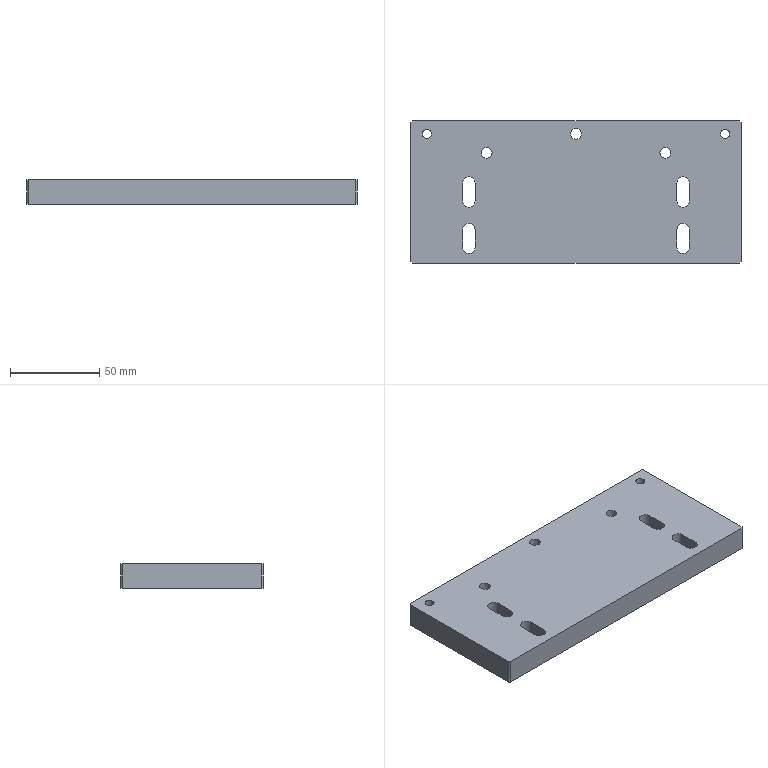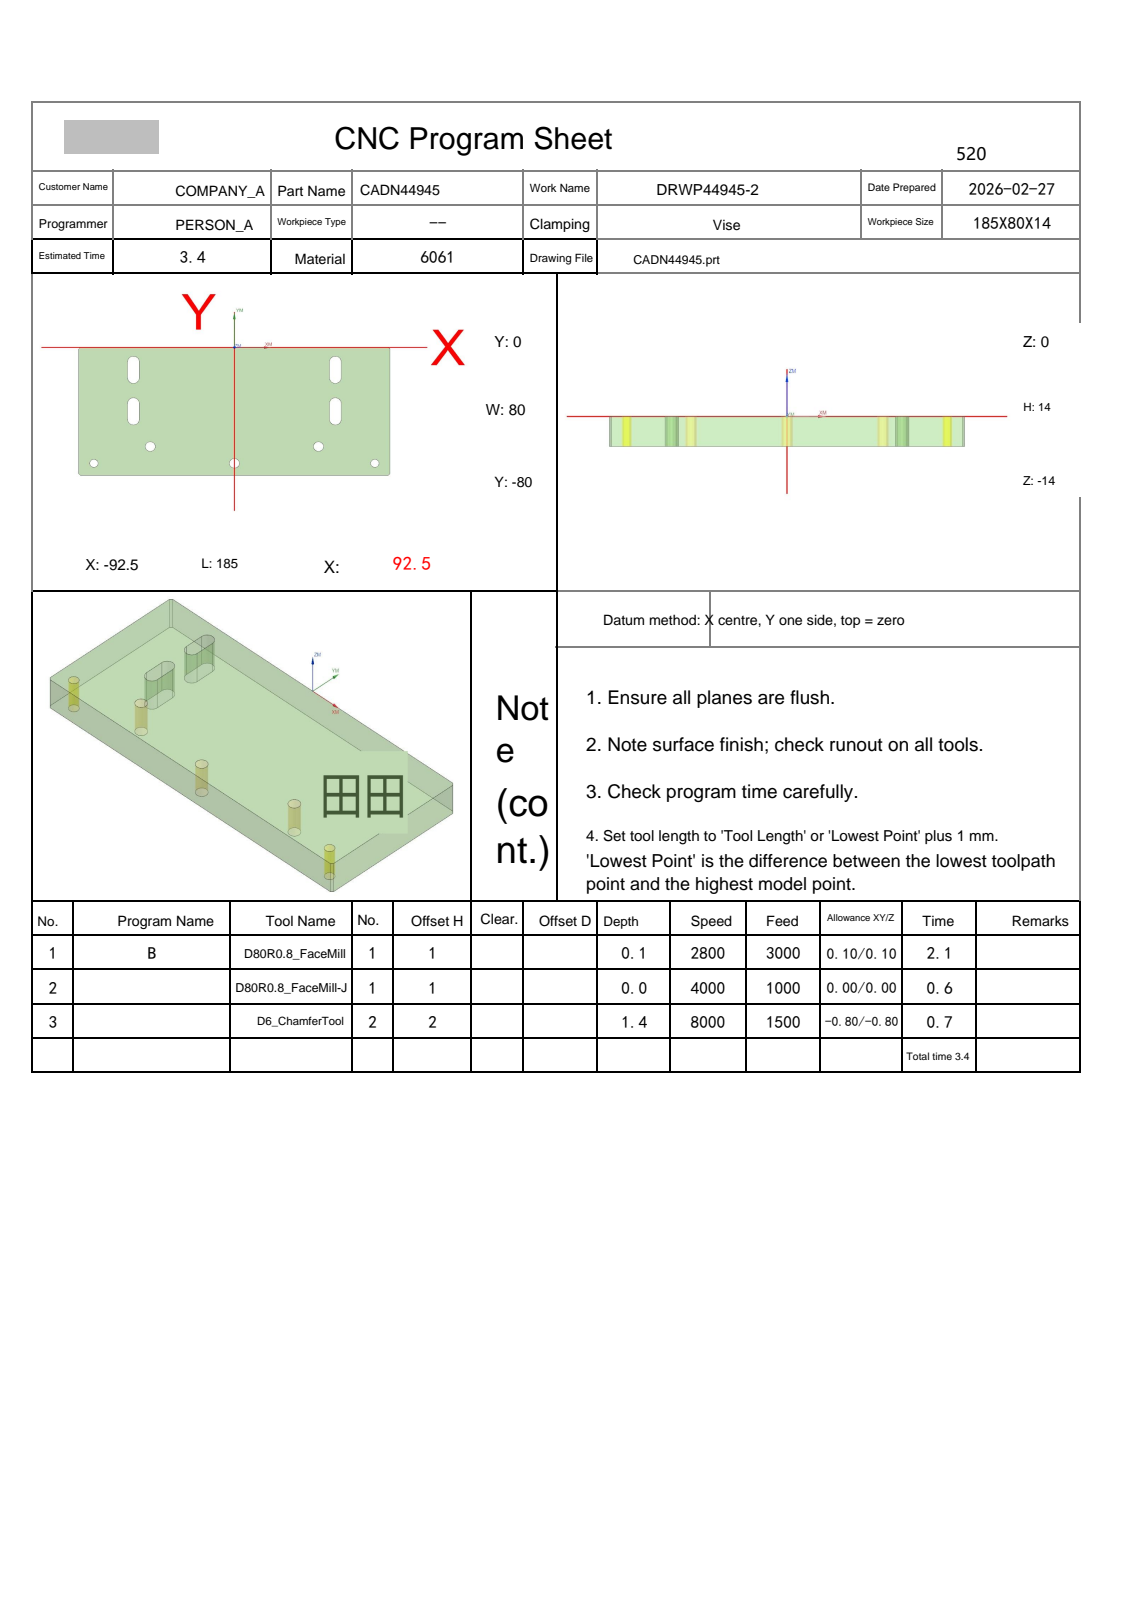NC program | NX | posted by the shop | part box 185 x 80 x 14 mm
Whole program:
%
O0001
(Machine time: 4.00 MIN)
(===Total Tool:2===)
(T1=D80R0.8-FaceMill D=80.  R=0.8  D-  H01 Z=-0.   )
(T2=D6_ChamferTool   D=6.   R=0.   D-  H02 Z=-1.4  )
G80 G90 G17 G49 G40
G91 G28 Z0
M01
N1 T01 M06
(D80R0.8-FaceMill  D=80. R=0.8 H=01 ce=0.10 di=0.10)
G00 G90 G54 X144.597 Y-56.097 M03 S2800
G43 H01 Z50.
M08
Z7.009
G01 Z5.009 F3000.
X132.597
X-125.397
G02 X-132.597 Y-48.897 I0.0 J7.2
G01 Y-39.263
G02 X-124.597 Y-31.263 I8. J0.0
G01 X132.597
X144.597
Z7.009
G00 Y-56.097
Z6.518
G01 Z4.518
X132.597
X-125.397
G02 X-132.597 Y-48.897 I0.0 J7.2
G01 Y-39.263
G02 X-124.597 Y-31.263 I8. J0.0
G01 X132.597
X144.597
Z6.518
G00 Y-56.097
Z6.027
G01 Z4.027
X132.597
X-125.397
G02 X-132.597 Y-48.897 I0.0 J7.2
G01 Y-39.263
G02 X-124.597 Y-31.263 I8. J0.0
G01 X132.597
X144.597
Z6.027
G00 Y-56.097
Z5.536
G01 Z3.536
X132.597
X-125.397
G02 X-132.597 Y-48.897 I0.0 J7.2
G01 Y-39.263
G02 X-124.597 Y-31.263 I8. J0.0
G01 X132.597
X144.597
Z5.536
G00 Y-56.097
Z5.045
G01 Z3.045
X132.597
X-125.397
G02 X-132.597 Y-48.897 I0.0 J7.2
G01 Y-39.263
G02 X-124.597 Y-31.263 I8. J0.0
G01 X132.597
X144.597
Z5.045
G00 Y-56.097
Z4.555
G01 Z2.555
X132.597
X-125.397
G02 X-132.597 Y-48.897 I0.0 J7.2
G01 Y-39.263
G02 X-124.597 Y-31.263 I8. J0.0
G01 X132.597
X144.597
Z4.555
G00 Y-56.097
Z4.064
G01 Z2.064
X132.597
X-125.397
G02 X-132.597 Y-48.897 I0.0 J7.2
G01 Y-39.263
G02 X-124.597 Y-31.263 I8. J0.0
G01 X132.597
X144.597
Z4.064
G00 Y-56.097
Z3.573
G01 Z1.573
X132.597
X-125.397
G02 X-132.597 Y-48.897 I0.0 J7.2
G01 Y-39.263
G02 X-124.597 Y-31.263 I8. J0.0
G01 X132.597
X144.597
Z3.573
G00 Y-56.097
Z3.082
G01 Z1.082
X132.597
X-125.397
G02 X-132.597 Y-48.897 I0.0 J7.2
G01 Y-39.263
G02 X-124.597 Y-31.263 I8. J0.0
G01 X132.597
X144.597
Z3.082
G00 Y-56.097
Z2.591
G01 Z.591
X132.597
X-125.397
G02 X-132.597 Y-48.897 I0.0 J7.2
G01 Y-39.263
G02 X-124.597 Y-31.263 I8. J0.0
G01 X132.597
X144.597
Z2.591
G00 Y-56.097
Z2.1
G01 Z.1
X132.597
X-125.397
G02 X-132.597 Y-48.897 I0.0 J7.2
G01 Y-39.263
G02 X-124.597 Y-31.263 I8. J0.0
G01 X132.597
X144.597
Z2.1
G00 Z50.
G91 G28 Z0.0
M05
M09
G91 G28 Z0.0
M01
N2 T01 M06
(D80R0.8-FaceMill-J  D=80. R=0.8 H=01 ce=0.00 di=0.00)
G00 G90 G54 X144.499 Y-55.999 M03 S4000
G43 H01 Z50.
M08
Z2.
G01 Z0.0 F1000.
X132.499
X-125.299
G02 X-132.499 Y-48.799 I0.0 J7.2
G01 Y-39.361
G02 X-124.499 Y-31.361 I8. J0.0
G01 X132.499
X144.499
Z2.
G00 Z50.
G91 G28 Z0.0
M05
M09
G91 G28 Z0.0
M01
N3 T02 M06
(D6_ChamferTool  D=6. R=0. H=02 ce=-0.80 di=-0.80)
G00 G90 G54 X-83.732 Y-71.63 M03 S8000
G43 H02 Z50.
M08
Z-.9
G01 Z-1.4 F600.
X-83.9 Y-71.
G03 X-85.4 Y-72.5 I0.0 J-1.5
X-83.5 Y-74.4 I1.9 J0.0
X-81.6 Y-72.5 I0.0 J1.9
X-83.5 Y-70.6 I-1.9 J0.0
X-85.4 Y-72.5 I0.0 J-1.9
X-83.9 Y-74. I1.5 J0.0
G01 X-83.732 Y-73.37
Z-.9
G00 Z50.
X83.268 Y-71.63
Z-.9
G01 Z-1.4
X83.1 Y-71.
G03 X81.6 Y-72.5 I0.0 J-1.5
X83.5 Y-74.4 I1.9 J0.0
X85.4 Y-72.5 I0.0 J1.9
X83.5 Y-70.6 I-1.9 J0.0
X81.6 Y-72.5 I0.0 J-1.9
X83.1 Y-74. I1.5 J0.0
G01 X83.268 Y-73.37
Z-.9
G00 Z50.
G00 G90 X.386 Y-81.227 M03 S6500
Z50.
Z.172
G01 Z-1.2 F1500.
G03 X.1 Y-81.027 I-1.286 J-1.532
G01 X.054 Y-80.997
X0.0 Y-81.
X-91.5
X-91.759 Y-80.966
X-92. Y-80.866
X-92.207 Y-80.707
X-93.207 Y-79.707
X-93.366 Y-79.5
X-93.466 Y-79.259
X-93.5 Y-79.
Y-1.
X-93.466 Y-.741
X-93.366 Y-.5
X-93.207 Y-.293
X-92.207 Y.707
X-92. Y.866
X-91.759 Y.966
X-91.5 Y1.
X91.5
X91.759 Y.966
X92. Y.866
X92.207 Y.707
X93.207 Y-.293
X93.366 Y-.5
X93.466 Y-.741
X93.5 Y-1.
Y-79.
X93.466 Y-79.259
X93.366 Y-79.5
X93.207 Y-79.707
X92.207 Y-80.707
X92. Y-80.866
X91.759 Y-80.966
X91.5 Y-81.
X0.0
X-.054 Y-80.997
X-.1 Y-81.027
G03 X-.386 Y-81.227 I1. J-1.732
G01 Z.172
G00 Z10.
X-84.815 Y-72.093
Z.284
G01 Z-1.2
G03 X-84.984 Y-72.398 I1.658 J-1.118
G01 X-85.009 Y-72.446
X-85. Y-72.5
G03 X-83.5 Y-74. I1.5 J0.0
X-82. Y-72.5 I0.0 J1.5
X-83.5 Y-71. I-1.5 J0.0
X-85. Y-72.5 I0.0 J-1.5
G01 X-85.009 Y-72.554
X-84.984 Y-72.602
G03 X-84.815 Y-72.907 I1.827 J.813
G01 Z.284
G00 Z10.
X-57.727 Y-14.386
Z.172
G01 Z-1.2
G03 X-57.527 Y-14.1 I-1.532 J1.286
G01 X-57.497 Y-14.054
X-57.5 Y-14.
Y-9.
G03 X-60. Y-6.5 I-2.5 J0.0
X-62.5 Y-9. I0.0 J-2.5
G01 Y-19.
G03 X-60. Y-21.5 I2.5 J0.0
X-57.5 Y-19. I0.0 J2.5
G01 Y-14.
X-57.497 Y-13.946
X-57.527 Y-13.9
G03 X-57.727 Y-13.614 I-1.732 J-1.
G01 Z.172
G00 Z10.
Y-40.386
Z.172
G01 Z-1.2
G03 X-57.527 Y-40.1 I-1.532 J1.286
G01 X-57.497 Y-40.054
X-57.5 Y-40.
Y-35.
G03 X-60. Y-32.5 I-2.5 J0.0
X-62.5 Y-35. I0.0 J-2.5
G01 Y-45.
G03 X-60. Y-47.5 I2.5 J0.0
X-57.5 Y-45. I0.0 J2.5
G01 Y-40.
X-57.497 Y-39.946
X-57.527 Y-39.9
G03 X-57.727 Y-39.614 I-1.732 J-1.
G01 Z.172
G00 Z10.
X-51.808 Y-61.596
Z.257
G01 Z-1.2
G03 X-51.982 Y-61.898 I1.638 J-1.147
G01 X-52.008 Y-61.946
X-52. Y-62.
G03 X-50. Y-64. I2. J0.0
X-48. Y-62. I0.0 J2.
X-50. Y-60. I-2. J0.0
X-51.97 Y-61.653 I0.0 J-2.
G01 X-52. Y-62.
X-52.008 Y-62.054
X-51.982 Y-62.102
G03 X-51.808 Y-62.404 I1.813 J.845
G01 Z.257
G00 Z10.
X-1.808 Y-72.096
Z.257
G01 Z-1.2
G03 X-1.982 Y-72.398 I1.638 J-1.147
G01 X-2.008 Y-72.446
X-2. Y-72.5
G03 X0.0 Y-74.5 I2. J0.0
X2. Y-72.5 I0.0 J2.
X0.0 Y-70.5 I-2. J0.0
X-1.97 Y-72.153 I0.0 J-2.
G01 X-2. Y-72.5
X-2.008 Y-72.554
X-1.982 Y-72.602
G03 X-1.808 Y-72.904 I1.813 J.845
G01 Z.257
G00 Z10.
X48.192 Y-61.596
Z.257
G01 Z-1.2
G03 X48.018 Y-61.898 I1.638 J-1.147
G01 X47.992 Y-61.946
X48. Y-62.
G03 X50. Y-64. I2. J0.0
X52. Y-62. I0.0 J2.
X50. Y-60. I-2. J0.0
X48.03 Y-61.653 I0.0 J-2.
G01 X48. Y-62.
X47.992 Y-62.054
X48.018 Y-62.102
G03 X48.192 Y-62.404 I1.813 J.845
G01 Z.257
G00 Z10.
X82.185 Y-72.093
Z.284
G01 Z-1.2
G03 X82.016 Y-72.398 I1.658 J-1.118
G01 X81.991 Y-72.446
X82. Y-72.5
G03 X83.5 Y-74. I1.5 J0.0
X85. Y-72.5 I0.0 J1.5
X83.5 Y-71. I-1.5 J0.0
X82. Y-72.5 I0.0 J-1.5
G01 X81.991 Y-72.554
X82.016 Y-72.602
G03 X82.185 Y-72.907 I1.827 J.813
G01 Z.284
G00 Z10.
X57.727 Y-39.614
Z.172
G01 Z-1.2
G03 X57.527 Y-39.9 I1.532 J-1.286
G01 X57.497 Y-39.946
X57.5 Y-40.
Y-45.
G03 X60. Y-47.5 I2.5 J0.0
X62.5 Y-45. I0.0 J2.5
G01 Y-35.
G03 X60. Y-32.5 I-2.5 J0.0
X57.5 Y-35. I0.0 J-2.5
G01 Y-40.
X57.497 Y-40.054
X57.527 Y-40.1
G03 X57.727 Y-40.386 I1.732 J1.
G01 Z.172
G00 Z10.
Y-13.614
Z.172
G01 Z-1.2
G03 X57.527 Y-13.9 I1.532 J-1.286
G01 X57.497 Y-13.946
X57.5 Y-14.
Y-19.
G03 X60. Y-21.5 I2.5 J0.0
X62.5 Y-19. I0.0 J2.5
G01 Y-9.
G03 X60. Y-6.5 I-2.5 J0.0
X57.5 Y-9. I0.0 J-2.5
G01 Y-14.
X57.497 Y-14.054
X57.527 Y-14.1
G03 X57.727 Y-14.386 I1.732 J1.
G01 Z.172
G00 Z50.
M05
M09
G91 G28 Z0.0
G91 G28 Y0.0
M30
%